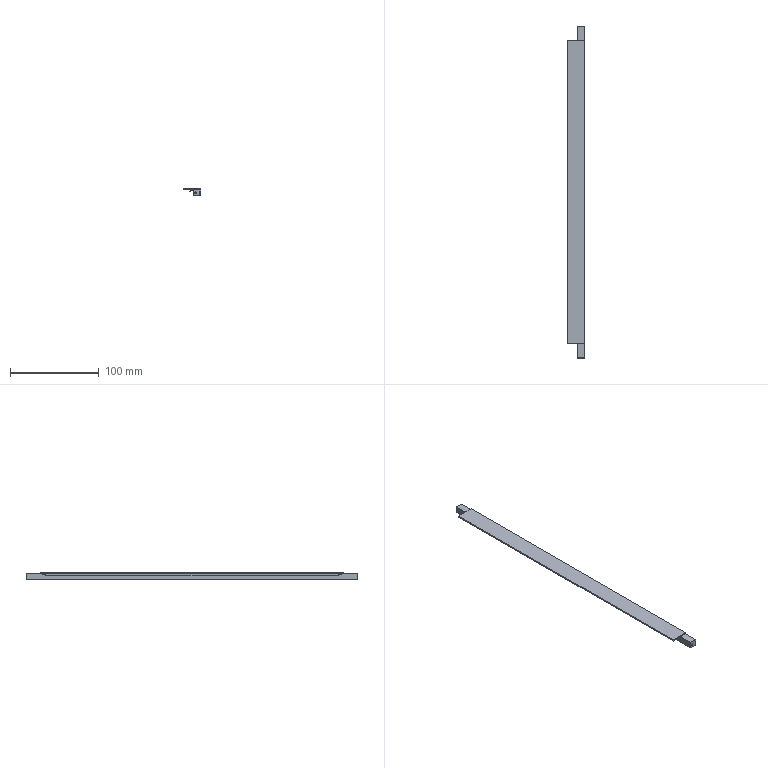Part | SolidWorks | features BaseBody 1 | 1 solid | 30 faces | box 20 x 374 x 9 mm | volume 32363 mm3 | plane 26 | cylinder 4 | commonest cylinder face diameters 2.076 x2 6 x2
STEP:
#1=CARTESIAN_POINT('',(265.038,187.,6.5));
#2=VERTEX_POINT('',#1);
#3=CARTESIAN_POINT('',(262.962,187.,6.5));
#4=VERTEX_POINT('',#3);
#5=CARTESIAN_POINT('',(264.,187.,6.5));
#6=DIRECTION('',(0.,1.,0.));
#7=DIRECTION('',(1.,0.,0.));
#8=AXIS2_PLACEMENT_3D('',#5,#6,#7);
#9=CIRCLE('',#8,1.038);
#10=EDGE_CURVE('',#2,#4,#9,.T.);
#11=ORIENTED_EDGE('',*,*,#10,.T.);
#12=CARTESIAN_POINT('',(262.962,-187.,6.5));
#13=VERTEX_POINT('',#12);
#14=CARTESIAN_POINT('',(262.962,18.7,6.5));
#15=DIRECTION('',(0.,-1.,0.));
#16=VECTOR('',#15,1000.);
#17=LINE('',#14,#16);
#18=EDGE_CURVE('',#4,#13,#17,.T.);
#19=ORIENTED_EDGE('',*,*,#18,.T.);
#20=CARTESIAN_POINT('',(265.038,-187.,6.5));
#21=VERTEX_POINT('',#20);
#22=CARTESIAN_POINT('',(264.,-187.,6.5));
#23=DIRECTION('',(0.,-1.,0.));
#24=DIRECTION('',(1.,0.,0.));
#25=AXIS2_PLACEMENT_3D('',#22,#23,#24);
#26=CIRCLE('',#25,1.038);
#27=EDGE_CURVE('',#13,#21,#26,.T.);
#28=ORIENTED_EDGE('',*,*,#27,.T.);
#29=CARTESIAN_POINT('',(265.038,18.7,6.5));
#30=DIRECTION('',(0.,-1.,0.));
#31=VECTOR('',#30,1000.);
#32=LINE('',#29,#31);
#33=EDGE_CURVE('',#2,#21,#32,.T.);
#34=ORIENTED_EDGE('',*,*,#33,.F.);
#35=EDGE_LOOP('',(#11,#19,#28,#34));
#36=FACE_OUTER_BOUND('',#35,.T.);
#37=CARTESIAN_POINT('',(264.,18.7,6.5));
#38=DIRECTION('',(0.,-1.,0.));
#39=DIRECTION('',(1.,0.,0.));
#40=AXIS2_PLACEMENT_3D('',#37,#38,#39);
#41=CYLINDRICAL_SURFACE('',#40,1.038);
#42=ADVANCED_FACE('',(#36),#41,.F.);
#43=CARTESIAN_POINT('',(250.,-171.,12.));
#44=VERTEX_POINT('',#43);
#45=CARTESIAN_POINT('',(250.,171.,12.));
#46=VERTEX_POINT('',#45);
#47=CARTESIAN_POINT('',(250.,-187.,12.));
#48=DIRECTION('',(0.,1.,0.));
#49=VECTOR('',#48,1000.);
#50=LINE('',#47,#49);
#51=EDGE_CURVE('',#44,#46,#50,.T.);
#52=ORIENTED_EDGE('',*,*,#51,.F.);
#53=CARTESIAN_POINT('',(270.,-171.,12.));
#54=VERTEX_POINT('',#53);
#55=CARTESIAN_POINT('',(270.,-171.,12.));
#56=DIRECTION('',(-1.,0.,0.));
#57=VECTOR('',#56,1000.);
#58=LINE('',#55,#57);
#59=EDGE_CURVE('',#54,#44,#58,.T.);
#60=ORIENTED_EDGE('',*,*,#59,.F.);
#61=CARTESIAN_POINT('',(270.,171.,12.));
#62=VERTEX_POINT('',#61);
#63=CARTESIAN_POINT('',(270.,-187.,12.));
#64=DIRECTION('',(0.,-1.,0.));
#65=VECTOR('',#64,1000.);
#66=LINE('',#63,#65);
#67=EDGE_CURVE('',#62,#54,#66,.T.);
#68=ORIENTED_EDGE('',*,*,#67,.F.);
#69=CARTESIAN_POINT('',(270.,171.,12.));
#70=DIRECTION('',(1.,0.,0.));
#71=VECTOR('',#70,1000.);
#72=LINE('',#69,#71);
#73=EDGE_CURVE('',#46,#62,#72,.T.);
#74=ORIENTED_EDGE('',*,*,#73,.F.);
#75=EDGE_LOOP('',(#52,#60,#68,#74));
#76=FACE_OUTER_BOUND('',#75,.T.);
#77=CARTESIAN_POINT('',(270.,-187.,12.));
#78=DIRECTION('',(0.,0.,-1.));
#79=DIRECTION('',(-1.,0.,0.));
#80=AXIS2_PLACEMENT_3D('',#77,#78,#79);
#81=PLANE('',#80);
#82=ADVANCED_FACE('',(#76),#81,.F.);
#83=CARTESIAN_POINT('',(262.,171.,10.5));
#84=VERTEX_POINT('',#83);
#85=CARTESIAN_POINT('',(250.,171.,10.5));
#86=VERTEX_POINT('',#85);
#87=CARTESIAN_POINT('',(250.,171.,10.5));
#88=DIRECTION('',(-1.,0.,0.));
#89=VECTOR('',#88,1000.);
#90=LINE('',#87,#89);
#91=EDGE_CURVE('',#84,#86,#90,.T.);
#92=ORIENTED_EDGE('',*,*,#91,.T.);
#93=CARTESIAN_POINT('',(250.,171.,12.));
#94=DIRECTION('',(0.,0.,1.));
#95=VECTOR('',#94,1000.);
#96=LINE('',#93,#95);
#97=EDGE_CURVE('',#86,#46,#96,.T.);
#98=ORIENTED_EDGE('',*,*,#97,.T.);
#99=ORIENTED_EDGE('',*,*,#73,.T.);
#100=CARTESIAN_POINT('',(270.,171.,10.5));
#101=VERTEX_POINT('',#100);
#102=CARTESIAN_POINT('',(270.,171.,12.));
#103=DIRECTION('',(0.,0.,-1.));
#104=VECTOR('',#103,1000.);
#105=LINE('',#102,#104);
#106=EDGE_CURVE('',#62,#101,#105,.T.);
#107=ORIENTED_EDGE('',*,*,#106,.T.);
#108=CARTESIAN_POINT('',(250.,171.,10.5));
#109=DIRECTION('',(-1.,0.,0.));
#110=VECTOR('',#109,1000.);
#111=LINE('',#108,#110);
#112=EDGE_CURVE('',#101,#84,#111,.T.);
#113=ORIENTED_EDGE('',*,*,#112,.T.);
#114=EDGE_LOOP('',(#92,#98,#99,#107,#113));
#115=FACE_OUTER_BOUND('',#114,.T.);
#116=CARTESIAN_POINT('',(250.,171.,12.));
#117=DIRECTION('',(0.,1.,0.));
#118=DIRECTION('',(0.,0.,1.));
#119=AXIS2_PLACEMENT_3D('',#116,#117,#118);
#120=PLANE('',#119);
#121=ADVANCED_FACE('',(#115),#120,.T.);
#122=CARTESIAN_POINT('',(250.,-171.,10.5));
#123=VERTEX_POINT('',#122);
#124=CARTESIAN_POINT('',(250.,-187.,10.5));
#125=DIRECTION('',(0.,1.,0.));
#126=VECTOR('',#125,1000.);
#127=LINE('',#124,#126);
#128=EDGE_CURVE('',#123,#86,#127,.T.);
#129=ORIENTED_EDGE('',*,*,#128,.F.);
#130=CARTESIAN_POINT('',(250.,-171.,12.));
#131=DIRECTION('',(0.,0.,-1.));
#132=VECTOR('',#131,1000.);
#133=LINE('',#130,#132);
#134=EDGE_CURVE('',#44,#123,#133,.T.);
#135=ORIENTED_EDGE('',*,*,#134,.F.);
#136=ORIENTED_EDGE('',*,*,#51,.T.);
#137=ORIENTED_EDGE('',*,*,#97,.F.);
#138=EDGE_LOOP('',(#129,#135,#136,#137));
#139=FACE_OUTER_BOUND('',#138,.T.);
#140=CARTESIAN_POINT('',(250.,-187.,12.));
#141=DIRECTION('',(1.,0.,0.));
#142=DIRECTION('',(0.,0.,-1.));
#143=AXIS2_PLACEMENT_3D('',#140,#141,#142);
#144=PLANE('',#143);
#145=ADVANCED_FACE('',(#139),#144,.F.);
#146=CARTESIAN_POINT('',(262.,-171.,10.5));
#147=VERTEX_POINT('',#146);
#148=CARTESIAN_POINT('',(270.,-171.,10.5));
#149=VERTEX_POINT('',#148);
#150=CARTESIAN_POINT('',(270.,-171.,10.5));
#151=DIRECTION('',(1.,0.,0.));
#152=VECTOR('',#151,1000.);
#153=LINE('',#150,#152);
#154=EDGE_CURVE('',#147,#149,#153,.T.);
#155=ORIENTED_EDGE('',*,*,#154,.T.);
#156=CARTESIAN_POINT('',(270.,-171.,12.));
#157=DIRECTION('',(0.,0.,1.));
#158=VECTOR('',#157,1000.);
#159=LINE('',#156,#158);
#160=EDGE_CURVE('',#149,#54,#159,.T.);
#161=ORIENTED_EDGE('',*,*,#160,.T.);
#162=ORIENTED_EDGE('',*,*,#59,.T.);
#163=ORIENTED_EDGE('',*,*,#134,.T.);
#164=CARTESIAN_POINT('',(270.,-171.,10.5));
#165=DIRECTION('',(1.,0.,0.));
#166=VECTOR('',#165,1000.);
#167=LINE('',#164,#166);
#168=EDGE_CURVE('',#123,#147,#167,.T.);
#169=ORIENTED_EDGE('',*,*,#168,.T.);
#170=EDGE_LOOP('',(#155,#161,#162,#163,#169));
#171=FACE_OUTER_BOUND('',#170,.T.);
#172=CARTESIAN_POINT('',(270.,-171.,12.));
#173=DIRECTION('',(0.,-1.,0.));
#174=DIRECTION('',(0.,0.,-1.));
#175=AXIS2_PLACEMENT_3D('',#172,#173,#174);
#176=PLANE('',#175);
#177=ADVANCED_FACE('',(#171),#176,.T.);
#178=CARTESIAN_POINT('',(270.,187.,10.5));
#179=VERTEX_POINT('',#178);
#180=CARTESIAN_POINT('',(270.,187.,8.5));
#181=VERTEX_POINT('',#180);
#182=CARTESIAN_POINT('',(270.,187.,3.));
#183=DIRECTION('',(0.,0.,-1.));
#184=VECTOR('',#183,1000.);
#185=LINE('',#182,#184);
#186=EDGE_CURVE('',#179,#181,#185,.T.);
#187=ORIENTED_EDGE('',*,*,#186,.F.);
#188=CARTESIAN_POINT('',(270.,-187.,10.5));
#189=DIRECTION('',(0.,1.,0.));
#190=VECTOR('',#189,1000.);
#191=LINE('',#188,#190);
#192=EDGE_CURVE('',#101,#179,#191,.T.);
#193=ORIENTED_EDGE('',*,*,#192,.F.);
#194=ORIENTED_EDGE('',*,*,#106,.F.);
#195=ORIENTED_EDGE('',*,*,#67,.T.);
#196=ORIENTED_EDGE('',*,*,#160,.F.);
#197=CARTESIAN_POINT('',(270.,-187.,10.5));
#198=VERTEX_POINT('',#197);
#199=CARTESIAN_POINT('',(270.,-187.,10.5));
#200=DIRECTION('',(0.,1.,0.));
#201=VECTOR('',#200,1000.);
#202=LINE('',#199,#201);
#203=EDGE_CURVE('',#198,#149,#202,.T.);
#204=ORIENTED_EDGE('',*,*,#203,.F.);
#205=CARTESIAN_POINT('',(270.,-187.,8.5));
#206=VERTEX_POINT('',#205);
#207=CARTESIAN_POINT('',(270.,-187.,3.));
#208=DIRECTION('',(0.,0.,1.));
#209=VECTOR('',#208,1000.);
#210=LINE('',#207,#209);
#211=EDGE_CURVE('',#206,#198,#210,.T.);
#212=ORIENTED_EDGE('',*,*,#211,.F.);
#213=CARTESIAN_POINT('',(270.,-187.,8.5));
#214=DIRECTION('',(0.,-1.,0.));
#215=VECTOR('',#214,1000.);
#216=LINE('',#213,#215);
#217=EDGE_CURVE('',#181,#206,#216,.T.);
#218=ORIENTED_EDGE('',*,*,#217,.F.);
#219=EDGE_LOOP('',(#187,#193,#194,#195,#196,#204,#212,#218));
#220=FACE_OUTER_BOUND('',#219,.T.);
#221=CARTESIAN_POINT('',(270.,-187.,3.));
#222=DIRECTION('',(-1.,0.,0.));
#223=DIRECTION('',(0.,0.,1.));
#224=AXIS2_PLACEMENT_3D('',#221,#222,#223);
#225=PLANE('',#224);
#226=ADVANCED_FACE('',(#220),#225,.F.);
#227=ORIENTED_EDGE('',*,*,#91,.F.);
#228=CARTESIAN_POINT('',(262.,168.,10.5));
#229=VERTEX_POINT('',#228);
#230=CARTESIAN_POINT('',(262.,-187.,10.5));
#231=DIRECTION('',(0.,1.,0.));
#232=VECTOR('',#231,1000.);
#233=LINE('',#230,#232);
#234=EDGE_CURVE('',#229,#84,#233,.T.);
#235=ORIENTED_EDGE('',*,*,#234,.F.);
#236=CARTESIAN_POINT('',(259.,165.,10.5));
#237=VERTEX_POINT('',#236);
#238=CARTESIAN_POINT('',(259.,168.,10.5));
#239=DIRECTION('',(0.,0.,1.));
#240=DIRECTION('',(1.,0.,0.));
#241=AXIS2_PLACEMENT_3D('',#238,#239,#240);
#242=CIRCLE('',#241,3.);
#243=EDGE_CURVE('',#237,#229,#242,.T.);
#244=ORIENTED_EDGE('',*,*,#243,.F.);
#245=CARTESIAN_POINT('',(257.3,165.,10.5));
#246=VERTEX_POINT('',#245);
#247=CARTESIAN_POINT('',(250.,165.,10.5));
#248=DIRECTION('',(1.,0.,0.));
#249=VECTOR('',#248,1000.);
#250=LINE('',#247,#249);
#251=EDGE_CURVE('',#246,#237,#250,.T.);
#252=ORIENTED_EDGE('',*,*,#251,.F.);
#253=CARTESIAN_POINT('',(257.3,-165.,10.5));
#254=VERTEX_POINT('',#253);
#255=CARTESIAN_POINT('',(257.3,-187.,10.5));
#256=DIRECTION('',(0.,1.,0.));
#257=VECTOR('',#256,1000.);
#258=LINE('',#255,#257);
#259=EDGE_CURVE('',#254,#246,#258,.T.);
#260=ORIENTED_EDGE('',*,*,#259,.F.);
#261=CARTESIAN_POINT('',(259.,-165.,10.5));
#262=VERTEX_POINT('',#261);
#263=CARTESIAN_POINT('',(259.,-165.,10.5));
#264=DIRECTION('',(-1.,0.,0.));
#265=VECTOR('',#264,1000.);
#266=LINE('',#263,#265);
#267=EDGE_CURVE('',#262,#254,#266,.T.);
#268=ORIENTED_EDGE('',*,*,#267,.F.);
#269=CARTESIAN_POINT('',(262.,-168.,10.5));
#270=VERTEX_POINT('',#269);
#271=CARTESIAN_POINT('',(259.,-168.,10.5));
#272=DIRECTION('',(0.,0.,1.));
#273=DIRECTION('',(1.,0.,0.));
#274=AXIS2_PLACEMENT_3D('',#271,#272,#273);
#275=CIRCLE('',#274,3.);
#276=EDGE_CURVE('',#270,#262,#275,.T.);
#277=ORIENTED_EDGE('',*,*,#276,.F.);
#278=CARTESIAN_POINT('',(262.,-187.,10.5));
#279=DIRECTION('',(0.,1.,0.));
#280=VECTOR('',#279,1000.);
#281=LINE('',#278,#280);
#282=EDGE_CURVE('',#147,#270,#281,.T.);
#283=ORIENTED_EDGE('',*,*,#282,.F.);
#284=ORIENTED_EDGE('',*,*,#168,.F.);
#285=ORIENTED_EDGE('',*,*,#128,.T.);
#286=EDGE_LOOP('',(#227,#235,#244,#252,#260,#268,#277,#283,#284,#285));
#287=FACE_OUTER_BOUND('',#286,.T.);
#288=CARTESIAN_POINT('',(250.,-187.,10.5));
#289=DIRECTION('',(0.,0.,1.));
#290=DIRECTION('',(1.,0.,0.));
#291=AXIS2_PLACEMENT_3D('',#288,#289,#290);
#292=PLANE('',#291);
#293=ADVANCED_FACE('',(#287),#292,.F.);
#294=ORIENTED_EDGE('',*,*,#192,.T.);
#295=CARTESIAN_POINT('',(262.,187.,10.5));
#296=VERTEX_POINT('',#295);
#297=CARTESIAN_POINT('',(260.,187.,10.5));
#298=DIRECTION('',(-1.,0.,0.));
#299=VECTOR('',#298,1000.);
#300=LINE('',#297,#299);
#301=EDGE_CURVE('',#179,#296,#300,.T.);
#302=ORIENTED_EDGE('',*,*,#301,.T.);
#303=CARTESIAN_POINT('',(262.,179.,10.5));
#304=DIRECTION('',(0.,-1.,0.));
#305=VECTOR('',#304,1000.);
#306=LINE('',#303,#305);
#307=EDGE_CURVE('',#296,#84,#306,.T.);
#308=ORIENTED_EDGE('',*,*,#307,.T.);
#309=ORIENTED_EDGE('',*,*,#112,.F.);
#310=EDGE_LOOP('',(#294,#302,#308,#309));
#311=FACE_OUTER_BOUND('',#310,.T.);
#312=CARTESIAN_POINT('',(260.,179.,10.5));
#313=DIRECTION('',(0.,0.,1.));
#314=DIRECTION('',(1.,0.,0.));
#315=AXIS2_PLACEMENT_3D('',#312,#313,#314);
#316=PLANE('',#315);
#317=ADVANCED_FACE('',(#311),#316,.T.);
#318=ORIENTED_EDGE('',*,*,#203,.T.);
#319=ORIENTED_EDGE('',*,*,#154,.F.);
#320=CARTESIAN_POINT('',(262.,-187.,10.5));
#321=VERTEX_POINT('',#320);
#322=CARTESIAN_POINT('',(262.,-179.,10.5));
#323=DIRECTION('',(0.,-1.,0.));
#324=VECTOR('',#323,1000.);
#325=LINE('',#322,#324);
#326=EDGE_CURVE('',#147,#321,#325,.T.);
#327=ORIENTED_EDGE('',*,*,#326,.T.);
#328=CARTESIAN_POINT('',(260.,-187.,10.5));
#329=DIRECTION('',(1.,0.,0.));
#330=VECTOR('',#329,1000.);
#331=LINE('',#328,#330);
#332=EDGE_CURVE('',#321,#198,#331,.T.);
#333=ORIENTED_EDGE('',*,*,#332,.T.);
#334=EDGE_LOOP('',(#318,#319,#327,#333));
#335=FACE_OUTER_BOUND('',#334,.T.);
#336=CARTESIAN_POINT('',(260.,-179.,10.5));
#337=DIRECTION('',(0.,0.,1.));
#338=DIRECTION('',(1.,0.,0.));
#339=AXIS2_PLACEMENT_3D('',#336,#337,#338);
#340=PLANE('',#339);
#341=ADVANCED_FACE('',(#335),#340,.T.);
#342=CARTESIAN_POINT('',(269.,-187.,8.5));
#343=VERTEX_POINT('',#342);
#344=CARTESIAN_POINT('',(270.,-187.,8.5));
#345=DIRECTION('',(-1.,0.,0.));
#346=VECTOR('',#345,1000.);
#347=LINE('',#344,#346);
#348=EDGE_CURVE('',#206,#343,#347,.T.);
#349=ORIENTED_EDGE('',*,*,#348,.T.);
#350=CARTESIAN_POINT('',(269.,187.,8.5));
#351=VERTEX_POINT('',#350);
#352=CARTESIAN_POINT('',(269.,-187.,8.5));
#353=DIRECTION('',(0.,1.,0.));
#354=VECTOR('',#353,1000.);
#355=LINE('',#352,#354);
#356=EDGE_CURVE('',#343,#351,#355,.T.);
#357=ORIENTED_EDGE('',*,*,#356,.T.);
#358=CARTESIAN_POINT('',(270.,187.,8.5));
#359=DIRECTION('',(1.,0.,0.));
#360=VECTOR('',#359,1000.);
#361=LINE('',#358,#360);
#362=EDGE_CURVE('',#351,#181,#361,.T.);
#363=ORIENTED_EDGE('',*,*,#362,.T.);
#364=ORIENTED_EDGE('',*,*,#217,.T.);
#365=EDGE_LOOP('',(#349,#357,#363,#364));
#366=FACE_OUTER_BOUND('',#365,.T.);
#367=CARTESIAN_POINT('',(270.,-187.,8.5));
#368=DIRECTION('',(0.,0.,-1.));
#369=DIRECTION('',(-1.,0.,0.));
#370=AXIS2_PLACEMENT_3D('',#367,#368,#369);
#371=PLANE('',#370);
#372=ADVANCED_FACE('',(#366),#371,.T.);
#373=ORIENTED_EDGE('',*,*,#10,.F.);
#374=CARTESIAN_POINT('',(264.,187.,6.5));
#375=DIRECTION('',(0.,1.,0.));
#376=DIRECTION('',(1.,0.,0.));
#377=AXIS2_PLACEMENT_3D('',#374,#375,#376);
#378=CIRCLE('',#377,1.038);
#379=EDGE_CURVE('',#4,#2,#378,.T.);
#380=ORIENTED_EDGE('',*,*,#379,.F.);
#381=EDGE_LOOP('',(#373,#380));
#382=FACE_BOUND('',#381,.T.);
#383=CARTESIAN_POINT('',(270.,187.,4.5));
#384=VERTEX_POINT('',#383);
#385=CARTESIAN_POINT('',(270.,187.,3.));
#386=VERTEX_POINT('',#385);
#387=CARTESIAN_POINT('',(270.,187.,3.));
#388=DIRECTION('',(0.,0.,-1.));
#389=VECTOR('',#388,1000.);
#390=LINE('',#387,#389);
#391=EDGE_CURVE('',#384,#386,#390,.T.);
#392=ORIENTED_EDGE('',*,*,#391,.T.);
#393=CARTESIAN_POINT('',(262.,187.,3.));
#394=VERTEX_POINT('',#393);
#395=CARTESIAN_POINT('',(260.,187.,3.));
#396=DIRECTION('',(1.,0.,0.));
#397=VECTOR('',#396,1000.);
#398=LINE('',#395,#397);
#399=EDGE_CURVE('',#394,#386,#398,.T.);
#400=ORIENTED_EDGE('',*,*,#399,.F.);
#401=CARTESIAN_POINT('',(262.,187.,7.5));
#402=DIRECTION('',(0.,0.,-1.));
#403=VECTOR('',#402,1000.);
#404=LINE('',#401,#403);
#405=EDGE_CURVE('',#296,#394,#404,.T.);
#406=ORIENTED_EDGE('',*,*,#405,.F.);
#407=ORIENTED_EDGE('',*,*,#301,.F.);
#408=ORIENTED_EDGE('',*,*,#186,.T.);
#409=ORIENTED_EDGE('',*,*,#362,.F.);
#410=CARTESIAN_POINT('',(269.,187.,7.));
#411=VERTEX_POINT('',#410);
#412=CARTESIAN_POINT('',(269.,187.,7.5));
#413=DIRECTION('',(0.,0.,1.));
#414=VECTOR('',#413,1000.);
#415=LINE('',#412,#414);
#416=EDGE_CURVE('',#411,#351,#415,.T.);
#417=ORIENTED_EDGE('',*,*,#416,.F.);
#418=CARTESIAN_POINT('',(270.,187.,7.));
#419=VERTEX_POINT('',#418);
#420=CARTESIAN_POINT('',(269.,187.,7.));
#421=DIRECTION('',(-1.,0.,0.));
#422=VECTOR('',#421,1000.);
#423=LINE('',#420,#422);
#424=EDGE_CURVE('',#419,#411,#423,.T.);
#425=ORIENTED_EDGE('',*,*,#424,.F.);
#426=CARTESIAN_POINT('',(270.,187.,6.));
#427=VERTEX_POINT('',#426);
#428=CARTESIAN_POINT('',(270.,187.,3.));
#429=DIRECTION('',(0.,0.,-1.));
#430=VECTOR('',#429,1000.);
#431=LINE('',#428,#430);
#432=EDGE_CURVE('',#419,#427,#431,.T.);
#433=ORIENTED_EDGE('',*,*,#432,.T.);
#434=CARTESIAN_POINT('',(269.,187.,6.));
#435=VERTEX_POINT('',#434);
#436=CARTESIAN_POINT('',(270.,187.,6.));
#437=DIRECTION('',(1.,0.,0.));
#438=VECTOR('',#437,1000.);
#439=LINE('',#436,#438);
#440=EDGE_CURVE('',#435,#427,#439,.T.);
#441=ORIENTED_EDGE('',*,*,#440,.F.);
#442=CARTESIAN_POINT('',(269.,187.,4.5));
#443=VERTEX_POINT('',#442);
#444=CARTESIAN_POINT('',(269.,187.,6.));
#445=DIRECTION('',(0.,0.,1.));
#446=VECTOR('',#445,1000.);
#447=LINE('',#444,#446);
#448=EDGE_CURVE('',#443,#435,#447,.T.);
#449=ORIENTED_EDGE('',*,*,#448,.F.);
#450=CARTESIAN_POINT('',(269.,187.,4.5));
#451=DIRECTION('',(-1.,0.,0.));
#452=VECTOR('',#451,1000.);
#453=LINE('',#450,#452);
#454=EDGE_CURVE('',#384,#443,#453,.T.);
#455=ORIENTED_EDGE('',*,*,#454,.F.);
#456=EDGE_LOOP('',(#392,#400,#406,#407,#408,#409,#417,#425,#433,#441,#449,#455));
#457=FACE_OUTER_BOUND('',#456,.T.);
#458=CARTESIAN_POINT('',(260.,187.,7.5));
#459=DIRECTION('',(0.,-1.,0.));
#460=DIRECTION('',(1.,0.,0.));
#461=AXIS2_PLACEMENT_3D('',#458,#459,#460);
#462=PLANE('',#461);
#463=ADVANCED_FACE('',(#382,#457),#462,.F.);
#464=CARTESIAN_POINT('',(264.,-187.,6.5));
#465=DIRECTION('',(0.,-1.,0.));
#466=DIRECTION('',(1.,0.,0.));
#467=AXIS2_PLACEMENT_3D('',#464,#465,#466);
#468=CIRCLE('',#467,1.038);
#469=EDGE_CURVE('',#21,#13,#468,.T.);
#470=ORIENTED_EDGE('',*,*,#469,.F.);
#471=ORIENTED_EDGE('',*,*,#27,.F.);
#472=EDGE_LOOP('',(#470,#471));
#473=FACE_BOUND('',#472,.T.);
#474=CARTESIAN_POINT('',(269.,-187.,6.));
#475=VERTEX_POINT('',#474);
#476=CARTESIAN_POINT('',(269.,-187.,4.5));
#477=VERTEX_POINT('',#476);
#478=CARTESIAN_POINT('',(269.,-187.,6.));
#479=DIRECTION('',(0.,0.,-1.));
#480=VECTOR('',#479,1000.);
#481=LINE('',#478,#480);
#482=EDGE_CURVE('',#475,#477,#481,.T.);
#483=ORIENTED_EDGE('',*,*,#482,.F.);
#484=CARTESIAN_POINT('',(270.,-187.,6.));
#485=VERTEX_POINT('',#484);
#486=CARTESIAN_POINT('',(270.,-187.,6.));
#487=DIRECTION('',(-1.,0.,0.));
#488=VECTOR('',#487,1000.);
#489=LINE('',#486,#488);
#490=EDGE_CURVE('',#485,#475,#489,.T.);
#491=ORIENTED_EDGE('',*,*,#490,.F.);
#492=CARTESIAN_POINT('',(270.,-187.,7.));
#493=VERTEX_POINT('',#492);
#494=CARTESIAN_POINT('',(270.,-187.,3.));
#495=DIRECTION('',(0.,0.,1.));
#496=VECTOR('',#495,1000.);
#497=LINE('',#494,#496);
#498=EDGE_CURVE('',#485,#493,#497,.T.);
#499=ORIENTED_EDGE('',*,*,#498,.T.);
#500=CARTESIAN_POINT('',(269.,-187.,7.));
#501=VERTEX_POINT('',#500);
#502=CARTESIAN_POINT('',(269.,-187.,7.));
#503=DIRECTION('',(1.,0.,0.));
#504=VECTOR('',#503,1000.);
#505=LINE('',#502,#504);
#506=EDGE_CURVE('',#501,#493,#505,.T.);
#507=ORIENTED_EDGE('',*,*,#506,.F.);
#508=CARTESIAN_POINT('',(269.,-187.,7.5));
#509=DIRECTION('',(0.,0.,-1.));
#510=VECTOR('',#509,1000.);
#511=LINE('',#508,#510);
#512=EDGE_CURVE('',#343,#501,#511,.T.);
#513=ORIENTED_EDGE('',*,*,#512,.F.);
#514=ORIENTED_EDGE('',*,*,#348,.F.);
#515=ORIENTED_EDGE('',*,*,#211,.T.);
#516=ORIENTED_EDGE('',*,*,#332,.F.);
#517=CARTESIAN_POINT('',(262.,-187.,3.));
#518=VERTEX_POINT('',#517);
#519=CARTESIAN_POINT('',(262.,-187.,7.5));
#520=DIRECTION('',(0.,0.,1.));
#521=VECTOR('',#520,1000.);
#522=LINE('',#519,#521);
#523=EDGE_CURVE('',#518,#321,#522,.T.);
#524=ORIENTED_EDGE('',*,*,#523,.F.);
#525=CARTESIAN_POINT('',(270.,-187.,3.));
#526=VERTEX_POINT('',#525);
#527=CARTESIAN_POINT('',(260.,-187.,3.));
#528=DIRECTION('',(-1.,0.,0.));
#529=VECTOR('',#528,1000.);
#530=LINE('',#527,#529);
#531=EDGE_CURVE('',#526,#518,#530,.T.);
#532=ORIENTED_EDGE('',*,*,#531,.F.);
#533=CARTESIAN_POINT('',(270.,-187.,4.5));
#534=VERTEX_POINT('',#533);
#535=CARTESIAN_POINT('',(270.,-187.,3.));
#536=DIRECTION('',(0.,0.,1.));
#537=VECTOR('',#536,1000.);
#538=LINE('',#535,#537);
#539=EDGE_CURVE('',#526,#534,#538,.T.);
#540=ORIENTED_EDGE('',*,*,#539,.T.);
#541=CARTESIAN_POINT('',(269.,-187.,4.5));
#542=DIRECTION('',(1.,0.,0.));
#543=VECTOR('',#542,1000.);
#544=LINE('',#541,#543);
#545=EDGE_CURVE('',#477,#534,#544,.T.);
#546=ORIENTED_EDGE('',*,*,#545,.F.);
#547=EDGE_LOOP('',(#483,#491,#499,#507,#513,#514,#515,#516,#524,#532,#540,#546));
#548=FACE_OUTER_BOUND('',#547,.T.);
#549=CARTESIAN_POINT('',(260.,-187.,7.5));
#550=DIRECTION('',(0.,1.,0.));
#551=DIRECTION('',(0.,0.,1.));
#552=AXIS2_PLACEMENT_3D('',#549,#550,#551);
#553=PLANE('',#552);
#554=ADVANCED_FACE('',(#473,#548),#553,.F.);
#555=ORIENTED_EDGE('',*,*,#523,.T.);
#556=ORIENTED_EDGE('',*,*,#326,.F.);
#557=ORIENTED_EDGE('',*,*,#282,.T.);
#558=CARTESIAN_POINT('',(262.,-168.,9.5));
#559=VERTEX_POINT('',#558);
#560=CARTESIAN_POINT('',(262.,-168.,9.5));
#561=DIRECTION('',(0.,0.,1.));
#562=VECTOR('',#561,1000.);
#563=LINE('',#560,#562);
#564=EDGE_CURVE('',#559,#270,#563,.T.);
#565=ORIENTED_EDGE('',*,*,#564,.F.);
#566=CARTESIAN_POINT('',(262.,168.,9.5));
#567=VERTEX_POINT('',#566);
#568=CARTESIAN_POINT('',(262.,-187.,9.5));
#569=DIRECTION('',(0.,-1.,0.));
#570=VECTOR('',#569,1000.);
#571=LINE('',#568,#570);
#572=EDGE_CURVE('',#567,#559,#571,.T.);
#573=ORIENTED_EDGE('',*,*,#572,.F.);
#574=CARTESIAN_POINT('',(262.,168.,9.5));
#575=DIRECTION('',(0.,0.,-1.));
#576=VECTOR('',#575,1000.);
#577=LINE('',#574,#576);
#578=EDGE_CURVE('',#229,#567,#577,.T.);
#579=ORIENTED_EDGE('',*,*,#578,.F.);
#580=ORIENTED_EDGE('',*,*,#234,.T.);
#581=ORIENTED_EDGE('',*,*,#307,.F.);
#582=ORIENTED_EDGE('',*,*,#405,.T.);
#583=CARTESIAN_POINT('',(262.,-187.,3.));
#584=DIRECTION('',(0.,1.,0.));
#585=VECTOR('',#584,1000.);
#586=LINE('',#583,#585);
#587=EDGE_CURVE('',#518,#394,#586,.T.);
#588=ORIENTED_EDGE('',*,*,#587,.F.);
#589=EDGE_LOOP('',(#555,#556,#557,#565,#573,#579,#580,#581,#582,#588));
#590=FACE_OUTER_BOUND('',#589,.T.);
#591=CARTESIAN_POINT('',(262.,-187.,9.5));
#592=DIRECTION('',(1.,0.,0.));
#593=DIRECTION('',(0.,0.,-1.));
#594=AXIS2_PLACEMENT_3D('',#591,#592,#593);
#595=PLANE('',#594);
#596=ADVANCED_FACE('',(#590),#595,.F.);
#597=CARTESIAN_POINT('',(259.,165.,9.5));
#598=VERTEX_POINT('',#597);
#599=CARTESIAN_POINT('',(259.,165.,10.5));
#600=DIRECTION('',(0.,0.,-1.));
#601=VECTOR('',#600,1000.);
#602=LINE('',#599,#601);
#603=EDGE_CURVE('',#237,#598,#602,.T.);
#604=ORIENTED_EDGE('',*,*,#603,.F.);
#605=ORIENTED_EDGE('',*,*,#243,.T.);
#606=ORIENTED_EDGE('',*,*,#578,.T.);
#607=CARTESIAN_POINT('',(259.,168.,9.5));
#608=DIRECTION('',(0.,0.,1.));
#609=DIRECTION('',(1.,0.,0.));
#610=AXIS2_PLACEMENT_3D('',#607,#608,#609);
#611=CIRCLE('',#610,3.);
#612=EDGE_CURVE('',#598,#567,#611,.T.);
#613=ORIENTED_EDGE('',*,*,#612,.F.);
#614=EDGE_LOOP('',(#604,#605,#606,#613));
#615=FACE_OUTER_BOUND('',#614,.T.);
#616=CARTESIAN_POINT('',(259.,168.,10.5));
#617=DIRECTION('',(0.,0.,1.));
#618=DIRECTION('',(1.,0.,0.));
#619=AXIS2_PLACEMENT_3D('',#616,#617,#618);
#620=CYLINDRICAL_SURFACE('',#619,3.);
#621=ADVANCED_FACE('',(#615),#620,.F.);
#622=CARTESIAN_POINT('',(257.3,-165.,8.5));
#623=VERTEX_POINT('',#622);
#624=CARTESIAN_POINT('',(257.3,165.,8.5));
#625=VERTEX_POINT('',#624);
#626=CARTESIAN_POINT('',(257.3,-187.,8.5));
#627=DIRECTION('',(0.,1.,0.));
#628=VECTOR('',#627,1000.);
#629=LINE('',#626,#628);
#630=EDGE_CURVE('',#623,#625,#629,.T.);
#631=ORIENTED_EDGE('',*,*,#630,.F.);
#632=CARTESIAN_POINT('',(257.3,-165.,10.5));
#633=DIRECTION('',(0.,0.,-1.));
#634=VECTOR('',#633,1000.);
#635=LINE('',#632,#634);
#636=EDGE_CURVE('',#254,#623,#635,.T.);
#637=ORIENTED_EDGE('',*,*,#636,.F.);
#638=ORIENTED_EDGE('',*,*,#259,.T.);
#639=CARTESIAN_POINT('',(257.3,165.,10.5));
#640=DIRECTION('',(0.,0.,1.));
#641=VECTOR('',#640,1000.);
#642=LINE('',#639,#641);
#643=EDGE_CURVE('',#625,#246,#642,.T.);
#644=ORIENTED_EDGE('',*,*,#643,.F.);
#645=EDGE_LOOP('',(#631,#637,#638,#644));
#646=FACE_OUTER_BOUND('',#645,.T.);
#647=CARTESIAN_POINT('',(257.3,-187.,10.5));
#648=DIRECTION('',(1.,0.,0.));
#649=DIRECTION('',(0.,0.,-1.));
#650=AXIS2_PLACEMENT_3D('',#647,#648,#649);
#651=PLANE('',#650);
#652=ADVANCED_FACE('',(#646),#651,.F.);
#653=ORIENTED_EDGE('',*,*,#564,.T.);
#654=ORIENTED_EDGE('',*,*,#276,.T.);
#655=CARTESIAN_POINT('',(259.,-165.,9.5));
#656=VERTEX_POINT('',#655);
#657=CARTESIAN_POINT('',(259.,-165.,10.5));
#658=DIRECTION('',(0.,0.,1.));
#659=VECTOR('',#658,1000.);
#660=LINE('',#657,#659);
#661=EDGE_CURVE('',#656,#262,#660,.T.);
#662=ORIENTED_EDGE('',*,*,#661,.F.);
#663=CARTESIAN_POINT('',(259.,-168.,9.5));
#664=DIRECTION('',(0.,0.,1.));
#665=DIRECTION('',(1.,0.,0.));
#666=AXIS2_PLACEMENT_3D('',#663,#664,#665);
#667=CIRCLE('',#666,3.);
#668=EDGE_CURVE('',#559,#656,#667,.T.);
#669=ORIENTED_EDGE('',*,*,#668,.F.);
#670=EDGE_LOOP('',(#653,#654,#662,#669));
#671=FACE_OUTER_BOUND('',#670,.T.);
#672=CARTESIAN_POINT('',(259.,-168.,10.5));
#673=DIRECTION('',(0.,0.,1.));
#674=DIRECTION('',(1.,0.,0.));
#675=AXIS2_PLACEMENT_3D('',#672,#673,#674);
#676=CYLINDRICAL_SURFACE('',#675,3.);
#677=ADVANCED_FACE('',(#671),#676,.F.);
#678=ORIENTED_EDGE('',*,*,#512,.T.);
#679=CARTESIAN_POINT('',(269.,-187.,7.));
#680=DIRECTION('',(0.,1.,0.));
#681=VECTOR('',#680,1000.);
#682=LINE('',#679,#681);
#683=EDGE_CURVE('',#501,#411,#682,.T.);
#684=ORIENTED_EDGE('',*,*,#683,.T.);
#685=ORIENTED_EDGE('',*,*,#416,.T.);
#686=ORIENTED_EDGE('',*,*,#356,.F.);
#687=EDGE_LOOP('',(#678,#684,#685,#686));
#688=FACE_OUTER_BOUND('',#687,.T.);
#689=CARTESIAN_POINT('',(269.,-187.,8.5));
#690=DIRECTION('',(1.,0.,0.));
#691=DIRECTION('',(0.,1.,0.));
#692=AXIS2_PLACEMENT_3D('',#689,#690,#691);
#693=PLANE('',#692);
#694=ADVANCED_FACE('',(#688),#693,.T.);
#695=ORIENTED_EDGE('',*,*,#18,.F.);
#696=ORIENTED_EDGE('',*,*,#379,.T.);
#697=ORIENTED_EDGE('',*,*,#33,.T.);
#698=ORIENTED_EDGE('',*,*,#469,.T.);
#699=EDGE_LOOP('',(#695,#696,#697,#698));
#700=FACE_OUTER_BOUND('',#699,.T.);
#701=CARTESIAN_POINT('',(264.,18.7,6.5));
#702=DIRECTION('',(0.,-1.,0.));
#703=DIRECTION('',(1.,0.,0.));
#704=AXIS2_PLACEMENT_3D('',#701,#702,#703);
#705=CYLINDRICAL_SURFACE('',#704,1.038);
#706=ADVANCED_FACE('',(#700),#705,.F.);
#707=CARTESIAN_POINT('',(270.,-187.,3.));
#708=DIRECTION('',(0.,1.,0.));
#709=VECTOR('',#708,1000.);
#710=LINE('',#707,#709);
#711=EDGE_CURVE('',#526,#386,#710,.T.);
#712=ORIENTED_EDGE('',*,*,#711,.F.);
#713=ORIENTED_EDGE('',*,*,#531,.T.);
#714=ORIENTED_EDGE('',*,*,#587,.T.);
#715=ORIENTED_EDGE('',*,*,#399,.T.);
#716=EDGE_LOOP('',(#712,#713,#714,#715));
#717=FACE_OUTER_BOUND('',#716,.T.);
#718=CARTESIAN_POINT('',(262.,-187.,3.));
#719=DIRECTION('',(0.,0.,1.));
#720=DIRECTION('',(1.,0.,0.));
#721=AXIS2_PLACEMENT_3D('',#718,#719,#720);
#722=PLANE('',#721);
#723=ADVANCED_FACE('',(#717),#722,.F.);
#724=ORIENTED_EDGE('',*,*,#612,.T.);
#725=ORIENTED_EDGE('',*,*,#572,.T.);
#726=ORIENTED_EDGE('',*,*,#668,.T.);
#727=CARTESIAN_POINT('',(258.8,-165.,9.5));
#728=VERTEX_POINT('',#727);
#729=CARTESIAN_POINT('',(258.8,-165.,9.5));
#730=DIRECTION('',(1.,0.,0.));
#731=VECTOR('',#730,1000.);
#732=LINE('',#729,#731);
#733=EDGE_CURVE('',#728,#656,#732,.T.);
#734=ORIENTED_EDGE('',*,*,#733,.F.);
#735=CARTESIAN_POINT('',(258.8,165.,9.5));
#736=VERTEX_POINT('',#735);
#737=CARTESIAN_POINT('',(258.8,-187.,9.5));
#738=DIRECTION('',(0.,-1.,0.));
#739=VECTOR('',#738,1000.);
#740=LINE('',#737,#739);
#741=EDGE_CURVE('',#736,#728,#740,.T.);
#742=ORIENTED_EDGE('',*,*,#741,.F.);
#743=CARTESIAN_POINT('',(258.8,165.,9.5));
#744=DIRECTION('',(-1.,0.,0.));
#745=VECTOR('',#744,1000.);
#746=LINE('',#743,#745);
#747=EDGE_CURVE('',#598,#736,#746,.T.);
#748=ORIENTED_EDGE('',*,*,#747,.F.);
#749=EDGE_LOOP('',(#724,#725,#726,#734,#742,#748));
#750=FACE_OUTER_BOUND('',#749,.T.);
#751=CARTESIAN_POINT('',(258.8,-187.,9.5));
#752=DIRECTION('',(0.,0.,1.));
#753=DIRECTION('',(1.,0.,0.));
#754=AXIS2_PLACEMENT_3D('',#751,#752,#753);
#755=PLANE('',#754);
#756=ADVANCED_FACE('',(#750),#755,.F.);
#757=CARTESIAN_POINT('',(258.8,165.,8.5));
#758=VERTEX_POINT('',#757);
#759=CARTESIAN_POINT('',(258.8,165.,10.5));
#760=DIRECTION('',(0.,0.,-1.));
#761=VECTOR('',#760,1000.);
#762=LINE('',#759,#761);
#763=EDGE_CURVE('',#736,#758,#762,.T.);
#764=ORIENTED_EDGE('',*,*,#763,.T.);
#765=CARTESIAN_POINT('',(250.,165.,8.5));
#766=DIRECTION('',(-1.,0.,0.));
#767=VECTOR('',#766,1000.);
#768=LINE('',#765,#767);
#769=EDGE_CURVE('',#758,#625,#768,.T.);
#770=ORIENTED_EDGE('',*,*,#769,.T.);
#771=ORIENTED_EDGE('',*,*,#643,.T.);
#772=ORIENTED_EDGE('',*,*,#251,.T.);
#773=ORIENTED_EDGE('',*,*,#603,.T.);
#774=ORIENTED_EDGE('',*,*,#747,.T.);
#775=EDGE_LOOP('',(#764,#770,#771,#772,#773,#774));
#776=FACE_OUTER_BOUND('',#775,.T.);
#777=CARTESIAN_POINT('',(250.,165.,10.5));
#778=DIRECTION('',(0.,1.,0.));
#779=DIRECTION('',(0.,0.,1.));
#780=AXIS2_PLACEMENT_3D('',#777,#778,#779);
#781=PLANE('',#780);
#782=ADVANCED_FACE('',(#776),#781,.T.);
#783=CARTESIAN_POINT('',(258.8,-165.,8.5));
#784=VERTEX_POINT('',#783);
#785=CARTESIAN_POINT('',(258.8,-187.,8.5));
#786=DIRECTION('',(0.,1.,0.));
#787=VECTOR('',#786,1000.);
#788=LINE('',#785,#787);
#789=EDGE_CURVE('',#784,#758,#788,.T.);
#790=ORIENTED_EDGE('',*,*,#789,.F.);
#791=CARTESIAN_POINT('',(257.3,-165.,8.5));
#792=DIRECTION('',(1.,0.,0.));
#793=VECTOR('',#792,1000.);
#794=LINE('',#791,#793);
#795=EDGE_CURVE('',#623,#784,#794,.T.);
#796=ORIENTED_EDGE('',*,*,#795,.F.);
#797=ORIENTED_EDGE('',*,*,#630,.T.);
#798=ORIENTED_EDGE('',*,*,#769,.F.);
#799=EDGE_LOOP('',(#790,#796,#797,#798));
#800=FACE_OUTER_BOUND('',#799,.T.);
#801=CARTESIAN_POINT('',(257.3,-187.,8.5));
#802=DIRECTION('',(0.,0.,1.));
#803=DIRECTION('',(1.,0.,0.));
#804=AXIS2_PLACEMENT_3D('',#801,#802,#803);
#805=PLANE('',#804);
#806=ADVANCED_FACE('',(#800),#805,.F.);
#807=ORIENTED_EDGE('',*,*,#661,.T.);
#808=ORIENTED_EDGE('',*,*,#267,.T.);
#809=ORIENTED_EDGE('',*,*,#636,.T.);
#810=ORIENTED_EDGE('',*,*,#795,.T.);
#811=CARTESIAN_POINT('',(258.8,-165.,10.5));
#812=DIRECTION('',(0.,0.,1.));
#813=VECTOR('',#812,1000.);
#814=LINE('',#811,#813);
#815=EDGE_CURVE('',#784,#728,#814,.T.);
#816=ORIENTED_EDGE('',*,*,#815,.T.);
#817=ORIENTED_EDGE('',*,*,#733,.T.);
#818=EDGE_LOOP('',(#807,#808,#809,#810,#816,#817));
#819=FACE_OUTER_BOUND('',#818,.T.);
#820=CARTESIAN_POINT('',(259.,-165.,10.5));
#821=DIRECTION('',(0.,-1.,0.));
#822=DIRECTION('',(0.,0.,-1.));
#823=AXIS2_PLACEMENT_3D('',#820,#821,#822);
#824=PLANE('',#823);
#825=ADVANCED_FACE('',(#819),#824,.T.);
#826=ORIENTED_EDGE('',*,*,#506,.T.);
#827=CARTESIAN_POINT('',(270.,-187.,7.));
#828=DIRECTION('',(0.,1.,0.));
#829=VECTOR('',#828,1000.);
#830=LINE('',#827,#829);
#831=EDGE_CURVE('',#493,#419,#830,.T.);
#832=ORIENTED_EDGE('',*,*,#831,.T.);
#833=ORIENTED_EDGE('',*,*,#424,.T.);
#834=ORIENTED_EDGE('',*,*,#683,.F.);
#835=EDGE_LOOP('',(#826,#832,#833,#834));
#836=FACE_OUTER_BOUND('',#835,.T.);
#837=CARTESIAN_POINT('',(269.,-187.,7.));
#838=DIRECTION('',(0.,0.,1.));
#839=DIRECTION('',(1.,0.,0.));
#840=AXIS2_PLACEMENT_3D('',#837,#838,#839);
#841=PLANE('',#840);
#842=ADVANCED_FACE('',(#836),#841,.T.);
#843=ORIENTED_EDGE('',*,*,#539,.F.);
#844=ORIENTED_EDGE('',*,*,#711,.T.);
#845=ORIENTED_EDGE('',*,*,#391,.F.);
#846=CARTESIAN_POINT('',(270.,-187.,4.5));
#847=DIRECTION('',(0.,1.,0.));
#848=VECTOR('',#847,1000.);
#849=LINE('',#846,#848);
#850=EDGE_CURVE('',#534,#384,#849,.T.);
#851=ORIENTED_EDGE('',*,*,#850,.F.);
#852=EDGE_LOOP('',(#843,#844,#845,#851));
#853=FACE_OUTER_BOUND('',#852,.T.);
#854=CARTESIAN_POINT('',(270.,-187.,3.));
#855=DIRECTION('',(-1.,0.,0.));
#856=DIRECTION('',(0.,0.,1.));
#857=AXIS2_PLACEMENT_3D('',#854,#855,#856);
#858=PLANE('',#857);
#859=ADVANCED_FACE('',(#853),#858,.F.);
#860=ORIENTED_EDGE('',*,*,#741,.T.);
#861=ORIENTED_EDGE('',*,*,#815,.F.);
#862=ORIENTED_EDGE('',*,*,#789,.T.);
#863=ORIENTED_EDGE('',*,*,#763,.F.);
#864=EDGE_LOOP('',(#860,#861,#862,#863));
#865=FACE_OUTER_BOUND('',#864,.T.);
#866=CARTESIAN_POINT('',(258.8,-187.,8.5));
#867=DIRECTION('',(-1.,0.,0.));
#868=DIRECTION('',(0.,0.,1.));
#869=AXIS2_PLACEMENT_3D('',#866,#867,#868);
#870=PLANE('',#869);
#871=ADVANCED_FACE('',(#865),#870,.F.);
#872=ORIENTED_EDGE('',*,*,#432,.F.);
#873=ORIENTED_EDGE('',*,*,#831,.F.);
#874=ORIENTED_EDGE('',*,*,#498,.F.);
#875=CARTESIAN_POINT('',(270.,-187.,6.));
#876=DIRECTION('',(0.,-1.,0.));
#877=VECTOR('',#876,1000.);
#878=LINE('',#875,#877);
#879=EDGE_CURVE('',#427,#485,#878,.T.);
#880=ORIENTED_EDGE('',*,*,#879,.F.);
#881=EDGE_LOOP('',(#872,#873,#874,#880));
#882=FACE_OUTER_BOUND('',#881,.T.);
#883=CARTESIAN_POINT('',(270.,-187.,3.));
#884=DIRECTION('',(-1.,0.,0.));
#885=DIRECTION('',(0.,0.,1.));
#886=AXIS2_PLACEMENT_3D('',#883,#884,#885);
#887=PLANE('',#886);
#888=ADVANCED_FACE('',(#882),#887,.F.);
#889=ORIENTED_EDGE('',*,*,#545,.T.);
#890=ORIENTED_EDGE('',*,*,#850,.T.);
#891=ORIENTED_EDGE('',*,*,#454,.T.);
#892=CARTESIAN_POINT('',(269.,-187.,4.5));
#893=DIRECTION('',(0.,-1.,0.));
#894=VECTOR('',#893,1000.);
#895=LINE('',#892,#894);
#896=EDGE_CURVE('',#443,#477,#895,.T.);
#897=ORIENTED_EDGE('',*,*,#896,.T.);
#898=EDGE_LOOP('',(#889,#890,#891,#897));
#899=FACE_OUTER_BOUND('',#898,.T.);
#900=CARTESIAN_POINT('',(269.,-187.,4.5));
#901=DIRECTION('',(0.,0.,1.));
#902=DIRECTION('',(1.,0.,0.));
#903=AXIS2_PLACEMENT_3D('',#900,#901,#902);
#904=PLANE('',#903);
#905=ADVANCED_FACE('',(#899),#904,.T.);
#906=ORIENTED_EDGE('',*,*,#490,.T.);
#907=CARTESIAN_POINT('',(269.,-187.,6.));
#908=DIRECTION('',(0.,1.,0.));
#909=VECTOR('',#908,1000.);
#910=LINE('',#907,#909);
#911=EDGE_CURVE('',#475,#435,#910,.T.);
#912=ORIENTED_EDGE('',*,*,#911,.T.);
#913=ORIENTED_EDGE('',*,*,#440,.T.);
#914=ORIENTED_EDGE('',*,*,#879,.T.);
#915=EDGE_LOOP('',(#906,#912,#913,#914));
#916=FACE_OUTER_BOUND('',#915,.T.);
#917=CARTESIAN_POINT('',(270.,-187.,6.));
#918=DIRECTION('',(0.,0.,-1.));
#919=DIRECTION('',(-1.,0.,0.));
#920=AXIS2_PLACEMENT_3D('',#917,#918,#919);
#921=PLANE('',#920);
#922=ADVANCED_FACE('',(#916),#921,.T.);
#923=ORIENTED_EDGE('',*,*,#482,.T.);
#924=ORIENTED_EDGE('',*,*,#896,.F.);
#925=ORIENTED_EDGE('',*,*,#448,.T.);
#926=ORIENTED_EDGE('',*,*,#911,.F.);
#927=EDGE_LOOP('',(#923,#924,#925,#926));
#928=FACE_OUTER_BOUND('',#927,.T.);
#929=CARTESIAN_POINT('',(269.,-187.,6.));
#930=DIRECTION('',(1.,0.,0.));
#931=DIRECTION('',(0.,1.,0.));
#932=AXIS2_PLACEMENT_3D('',#929,#930,#931);
#933=PLANE('',#932);
#934=ADVANCED_FACE('',(#928),#933,.T.);
#935=CLOSED_SHELL('',(#42,#82,#121,#145,#177,#226,#293,#317,#341,#372,#463,#554,#596,#621,#652,#677,#694,#706,#723,#756,#782,#806,#825,#842,#859,#871,#888,#905,#922,#934));
#936=MANIFOLD_SOLID_BREP('',#935);
#937=CARTESIAN_POINT('',(0.,0.,0.));
#938=DIRECTION('',(0.,0.,1.));
#939=DIRECTION('',(1.,0.,0.));
#940=AXIS2_PLACEMENT_3D('',#937,#938,#939);
#941=(LENGTH_UNIT()NAMED_UNIT(*)SI_UNIT(.MILLI.,.METRE.));
#942=UNCERTAINTY_MEASURE_WITH_UNIT(LENGTH_MEASURE(0.00001),#941,'','');
#943=(NAMED_UNIT(*)PLANE_ANGLE_UNIT()SI_UNIT($,.RADIAN.));
#944=(NAMED_UNIT(*)SI_UNIT($,.STERADIAN.)SOLID_ANGLE_UNIT());
#945=(GEOMETRIC_REPRESENTATION_CONTEXT(3)GLOBAL_UNCERTAINTY_ASSIGNED_CONTEXT((#942))GLOBAL_UNIT_ASSIGNED_CONTEXT((#941,#943,#944))REPRESENTATION_CONTEXT('',''));
#946=ADVANCED_BREP_SHAPE_REPRESENTATION('',(#936,#940),#945);